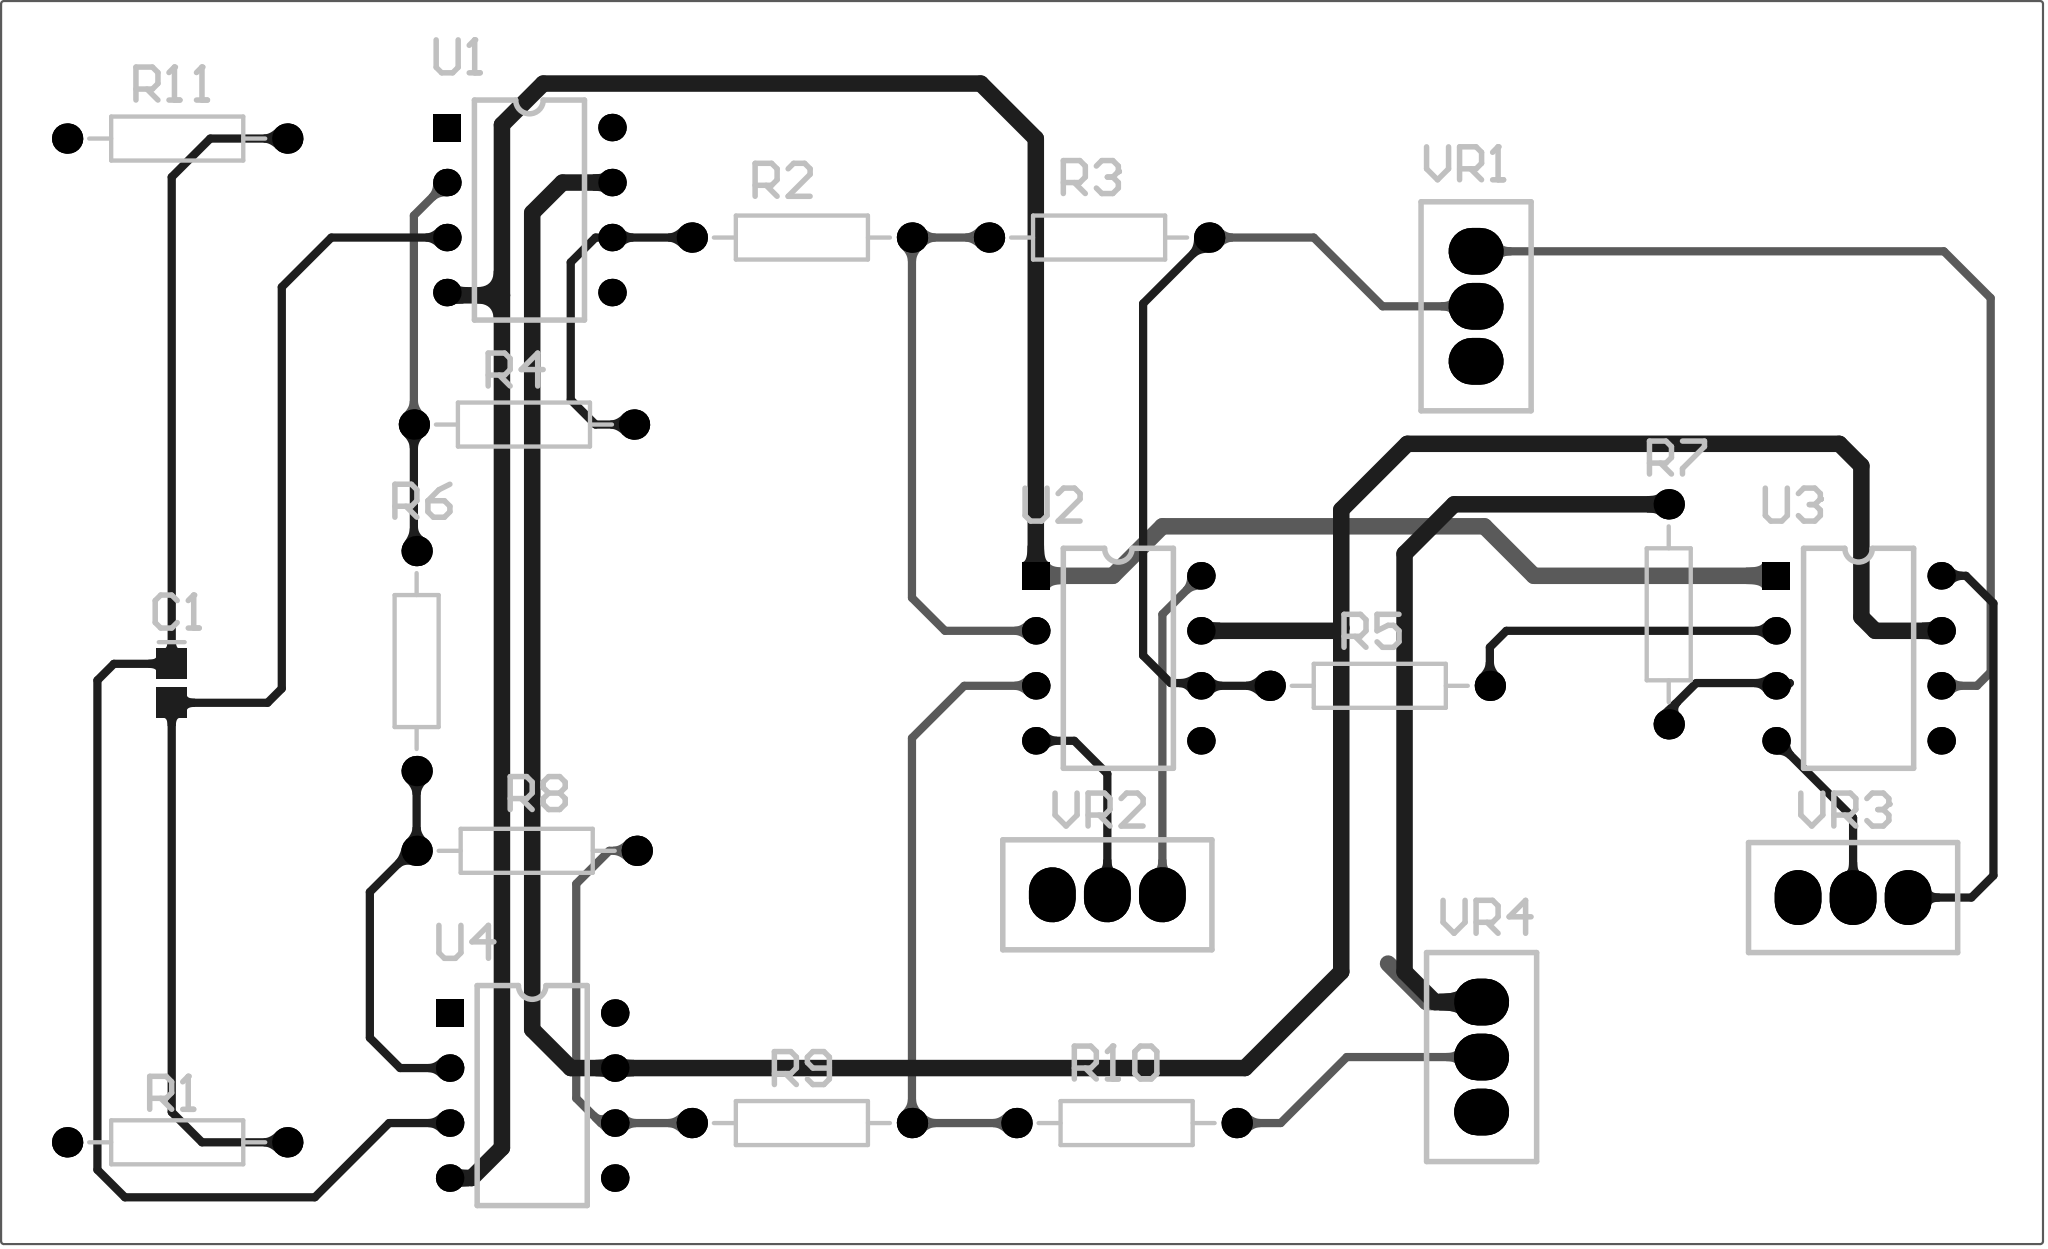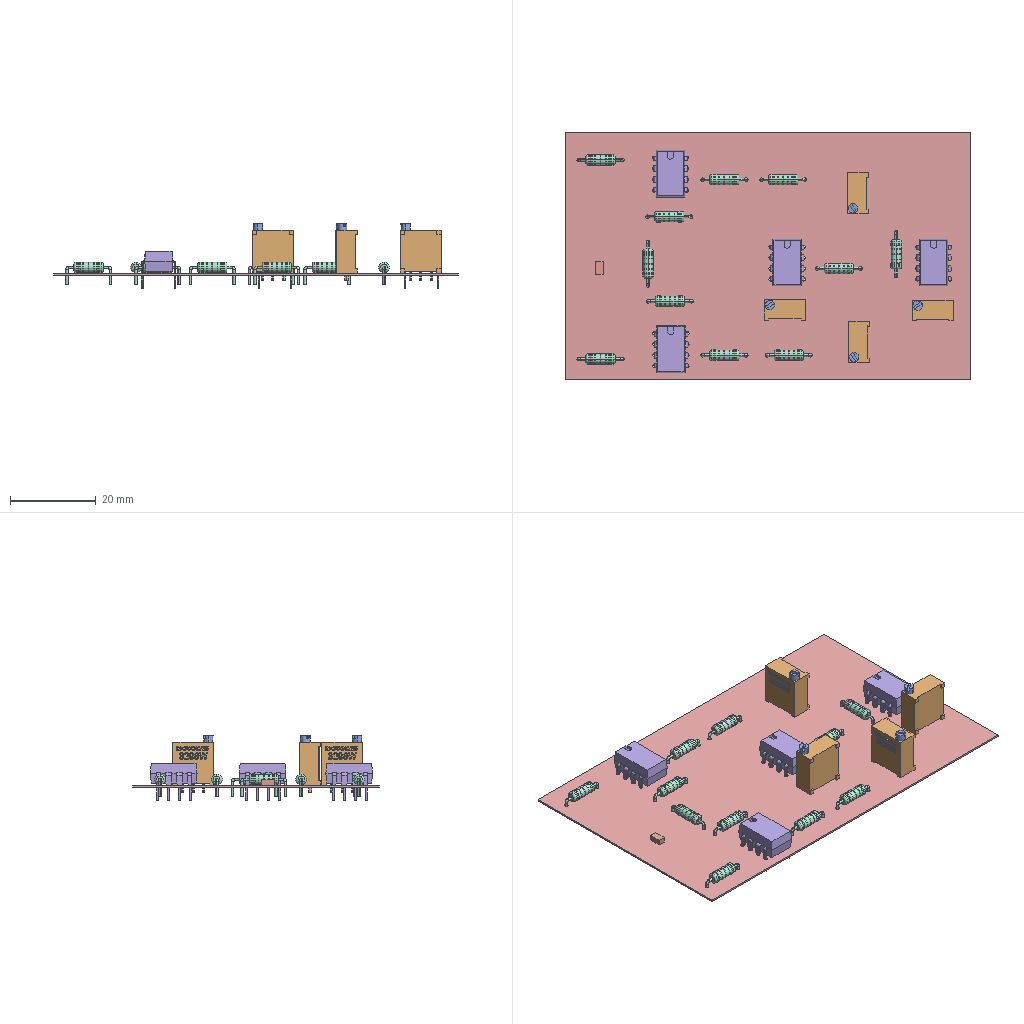Circuit board layout | Altium Designer | box 94.2 x 57.4 x 15 mm
Layer stack:
# Altium Designer layer stack of  (unit mm; dielectric type: 0 none, 1 core, 2 prepreg, 3 surface material)
index,name,kind,layer,copper_thickness_mm,dielectric_type,dielectric_thickness_mm,dielectric_material,dielectric_constant
0,Top Paste,other,,,,,,
1,Top Overlay,other,,,,,,
2,Top Solder,dielectric,,,3,0.0102,Solder Resist,3.5
3,Top Layer,copper,Top Layer,0.0356,,,,
4,Dielectric 1,dielectric,,,0,0.32,FR-4,4.8
5,Bottom Layer,copper,Bottom Layer,0.0356,,,,
6,Bottom Solder,dielectric,,,3,0.0102,Solder Resist,3.5
7,Bottom Overlay,other,,,,,,
8,Bottom Paste,other,,,,,,
# drill layer pairs: low layer,high layer
drill_pair,Top Layer,Bottom Layer
Part placement:
Designator,Comment,Layer,Footprint,Center-X(mm),Center-Y(mm),Rotation
VR4,20K,TopLayer,3296W,113.284,33.909,270
VR3,20K,TopLayer,3296W,130.429,41.275,180
VR2,20K,TopLayer,3296W,96.012,41.402,180
VR1,100K,TopLayer,3296W,113.03,68.58,270
U4,OP07AH,TopLayer,DIP8,69.469,32.131,0
U3,OP07AH,TopLayer,DIP8,130.683,52.324,0
U2,OP07AH,TopLayer,DIP8,96.52,52.324,0
U1,OP07AH,TopLayer,DIP8,69.342,73.025,0
R11,200K,TopLayer,AXIAL0.4,53.086,76.327,360
R10,91K,TopLayer,AXIAL0.4,96.901,30.861,360
R9,10K,TopLayer,AXIAL0.4,81.915,30.861,360
R8,100K,TopLayer,AXIAL0.4,69.215,43.434,360
R7,10K,TopLayer,AXIAL0.4,121.92,54.356,270
R6,51K,TopLayer,AXIAL0.4,64.135,52.197,90
R5,10K,TopLayer,AXIAL0.4,108.585,51.054,360
R4,100K,TopLayer,AXIAL0.4,69.088,63.119,360
R3,39K,TopLayer,AXIAL0.4,95.631,71.755,360
R2,10K,TopLayer,AXIAL0.4,81.915,71.755,360
R1,200K,TopLayer,AXIAL0.4,53.086,29.972,360
C1,0.05UF,TopLayer,C2512,52.832,51.17,270
Pad and via stacks:
# Altium Designer via and pad stacks of  (unit mm). Each distinct definition once, with the count of objects using it.
# via: kind,start_layer,end_layer,hole_mm,diameter_mm,mode(0 simple;1 top-mid-bottom;2 full stack),diameter_per_layer,count,example_net
# pad: kind,layer,hole_mm,hole_type(0 round;1 square;2 slot),plating,top_size,top_shape(1 round;2 rect;3 octagon;9 rounded rect),mid_size,bottom_size,mode,footprint,size_per_layer,count,example
pad,Top Layer,0,0,plated,1.4x1.4,2,1.4x1.4,1.4x1.4,0,C2512,,2,C1.1
pad,Multi-Layer,0.8128,0,plated,1.27x1.27,1,1.27x1.27,1.27x1.27,0,DIP8,,28,U1.8
pad,Multi-Layer,0.8128,0,plated,1.27x1.27,2,1.27x1.27,1.27x1.27,0,DIP8,,4,U1.1
pad,Multi-Layer,0.85,0,plated,1.4x1.4,1,1.4x1.4,1.4x1.4,0,AXIAL0.4,,22,R1.2
pad,Multi-Layer,0.889,0,plated,2.159x2.54,1,2.159x2.54,2.159x2.54,0,3296W,,12,VR1.3
Design rules, without the lines most boards share:
# Altium Designer design rules of  (exported by Altium Designer, unit mm)
# columns: name | kind | enabled | priority | scope1 | scope2 | descriptor | typed fields (field=value)
SilkToSilkClearance | 55 | enabled | 1 | All | All | Silk to Silk (Clearance=0mil) (All),(All) |
SilkToSolderMaskClearance | 54 | enabled | 1 | IsPad | All | Silk To Solder Mask (Clearance=0mil) (IsPad),(All) |
MinimumSolderMaskSliver | 53 | enabled | 1 | All | All | Minimum Solder Mask Sliver (Gap=0mil) (All),(All) |
HoleToHoleClearance | 52 | enabled | 1 | All | All | Hole To Hole Clearance (Gap=10mil) (All),(All) | gap=0.254
DiffPairsRouting | 51 | enabled | 1 | All | All | Differential Pairs Uncoupled Length using the Gap Constraints (Min=10mil) (Max=10mil) (Prefered=10mil)  and Width Constraints (Min=15mil) (Max=15mil) (Prefered=15mil) (All) |
HoleSize | 42 | enabled | 1 | All | All | Hole Size Constraint (Min=1mil) (Max=9999mil) (All) |
SolderMaskExpansion | 13 | enabled | 1 | All | All | Solder Mask Expansion (Expansion =4mil) (All) | expansion=0.1016
PasteMaskExpansion | 14 | enabled | 1 | All | All | Paste Mask Expansion (Expansion =0mil) (All) | expansion=0
RoutingVias | 11 | enabled | 1 | All | All | Routing Via (MinHoleWidth=28mil) (MaxHoleWidth=28mil) (PreferredHoleWidth=28mil) (MinWidth=50mil) (MaxWidth=50mil) (PreferedWidth=50mil) (All) | via_min_hole=0.7112 via_max_hole=0.7112 via_preferred_diameter=1.27 via_preferred_hole=0.7112
Width | 2 | enabled | 1 | All | All | Width Constraint (Min=10mil) (Max=30mil) (Preferred=10mil) (All) |
PolygonConnect | 20 | enabled | 1 | All | All | Polygon Connect Rule(Relief Connect )(Conductor Width=10mil) (Relief Angle=90 Angle) (Entries=4) (Air Gap Width=10mil) (All),(All) | connect_style(0=relief,1=direct,2=none)=0 relief_conductor_width=0.254 relief_entries=4
PlaneConnect | 6 | enabled | 1 | All | All | Power Plane Connect Rule(Relief Connect )(Expansion=20mil) (Conductor Width=10mil) (Air Gap=10mil) (Entries=4) (All) | relief_conductor_width=0.254 relief_entries=4 relief_expansion=0.508
Clearance | 0 | enabled | 1 | All | All | Clearance Constraint (Gap=10mil) (All),(All) | gap=0.254
Classes set for this board:
# Altium Designer classes of  (member kind: 0 net, 1 component, 2 from-to, 3 pad, 4 layer, 5 differential pair, 6 design channel, 7 polygon, 8 structure, 9 xSignal)
# columns: class name | member kind | superclass | members
Sheet1 | 1 | no | C1; R1; R2; R3; R4; R5; R6; R7; R8; R9; R10; R11; U1; U2; U3; U4; VR1; VR2; VR3; VR4;